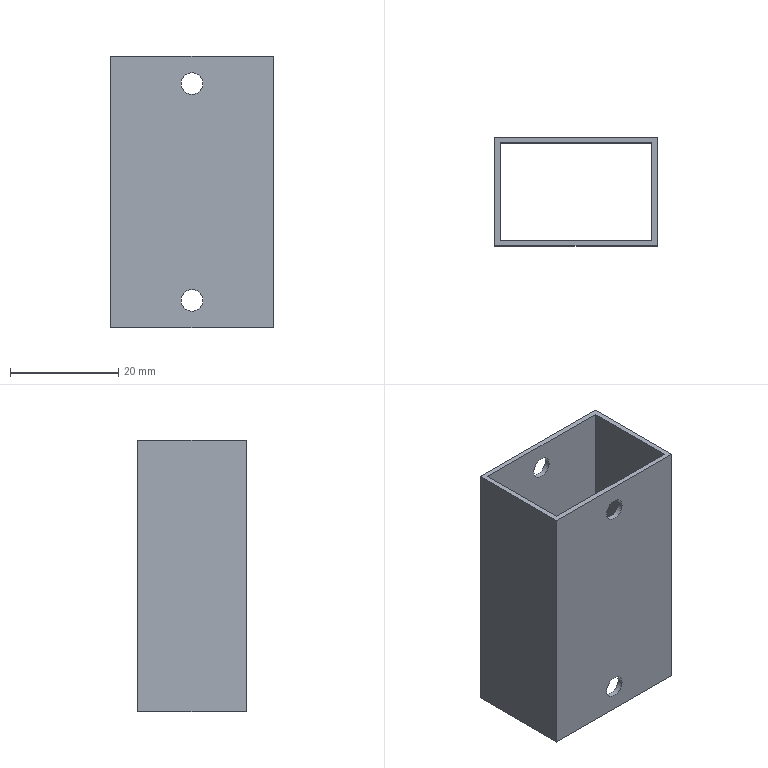Part | SolidWorks | features BaseBody 1 | 1 solid | 18 faces | box 30 x 20 x 50 mm | volume 4750 mm3 | plane 10 | cylinder 8 | commonest cylinder face diameters 4 x8
STEP:
#1=CARTESIAN_POINT('',(-2.,-10.,-20.));
#2=VERTEX_POINT('',#1);
#3=CARTESIAN_POINT('',(2.,-10.,-20.));
#4=VERTEX_POINT('',#3);
#5=CARTESIAN_POINT('',(0.,-10.,-20.));
#6=DIRECTION('',(0.,-1.,0.));
#7=DIRECTION('',(-1.,0.,0.));
#8=AXIS2_PLACEMENT_3D('',#5,#6,#7);
#9=CIRCLE('',#8,2.);
#10=EDGE_CURVE('',#2,#4,#9,.T.);
#11=ORIENTED_EDGE('',*,*,#10,.T.);
#12=CARTESIAN_POINT('',(2.,-9.,-20.));
#13=VERTEX_POINT('',#12);
#14=CARTESIAN_POINT('',(2.,-20.,-20.));
#15=DIRECTION('',(0.,1.,0.));
#16=VECTOR('',#15,1000.);
#17=LINE('',#14,#16);
#18=EDGE_CURVE('',#4,#13,#17,.T.);
#19=ORIENTED_EDGE('',*,*,#18,.T.);
#20=CARTESIAN_POINT('',(-2.,-9.,-20.));
#21=VERTEX_POINT('',#20);
#22=CARTESIAN_POINT('',(0.,-9.,-20.));
#23=DIRECTION('',(0.,-1.,0.));
#24=DIRECTION('',(-1.,0.,0.));
#25=AXIS2_PLACEMENT_3D('',#22,#23,#24);
#26=CIRCLE('',#25,2.);
#27=EDGE_CURVE('',#21,#13,#26,.T.);
#28=ORIENTED_EDGE('',*,*,#27,.F.);
#29=CARTESIAN_POINT('',(-2.,-20.,-20.));
#30=DIRECTION('',(0.,1.,0.));
#31=VECTOR('',#30,1000.);
#32=LINE('',#29,#31);
#33=EDGE_CURVE('',#2,#21,#32,.T.);
#34=ORIENTED_EDGE('',*,*,#33,.F.);
#35=EDGE_LOOP('',(#11,#19,#28,#34));
#36=FACE_OUTER_BOUND('',#35,.T.);
#37=CARTESIAN_POINT('',(0.,-20.,-20.));
#38=DIRECTION('',(0.,1.,0.));
#39=DIRECTION('',(-1.,0.,0.));
#40=AXIS2_PLACEMENT_3D('',#37,#38,#39);
#41=CYLINDRICAL_SURFACE('',#40,2.);
#42=ADVANCED_FACE('',(#36),#41,.F.);
#43=CARTESIAN_POINT('',(-2.,-10.,20.));
#44=VERTEX_POINT('',#43);
#45=CARTESIAN_POINT('',(2.,-10.,20.));
#46=VERTEX_POINT('',#45);
#47=CARTESIAN_POINT('',(0.,-10.,20.));
#48=DIRECTION('',(0.,-1.,0.));
#49=DIRECTION('',(-1.,0.,0.));
#50=AXIS2_PLACEMENT_3D('',#47,#48,#49);
#51=CIRCLE('',#50,2.);
#52=EDGE_CURVE('',#44,#46,#51,.T.);
#53=ORIENTED_EDGE('',*,*,#52,.T.);
#54=CARTESIAN_POINT('',(2.,-9.,20.));
#55=VERTEX_POINT('',#54);
#56=CARTESIAN_POINT('',(2.,-20.,20.));
#57=DIRECTION('',(0.,1.,0.));
#58=VECTOR('',#57,1000.);
#59=LINE('',#56,#58);
#60=EDGE_CURVE('',#46,#55,#59,.T.);
#61=ORIENTED_EDGE('',*,*,#60,.T.);
#62=CARTESIAN_POINT('',(-2.,-9.,20.));
#63=VERTEX_POINT('',#62);
#64=CARTESIAN_POINT('',(0.,-9.,20.));
#65=DIRECTION('',(0.,-1.,0.));
#66=DIRECTION('',(-1.,0.,0.));
#67=AXIS2_PLACEMENT_3D('',#64,#65,#66);
#68=CIRCLE('',#67,2.);
#69=EDGE_CURVE('',#63,#55,#68,.T.);
#70=ORIENTED_EDGE('',*,*,#69,.F.);
#71=CARTESIAN_POINT('',(-2.,-20.,20.));
#72=DIRECTION('',(0.,1.,0.));
#73=VECTOR('',#72,1000.);
#74=LINE('',#71,#73);
#75=EDGE_CURVE('',#44,#63,#74,.T.);
#76=ORIENTED_EDGE('',*,*,#75,.F.);
#77=EDGE_LOOP('',(#53,#61,#70,#76));
#78=FACE_OUTER_BOUND('',#77,.T.);
#79=CARTESIAN_POINT('',(0.,-20.,20.));
#80=DIRECTION('',(0.,1.,0.));
#81=DIRECTION('',(-1.,0.,0.));
#82=AXIS2_PLACEMENT_3D('',#79,#80,#81);
#83=CYLINDRICAL_SURFACE('',#82,2.);
#84=ADVANCED_FACE('',(#78),#83,.F.);
#85=CARTESIAN_POINT('',(2.,9.,-20.));
#86=VERTEX_POINT('',#85);
#87=CARTESIAN_POINT('',(-2.,9.,-20.));
#88=VERTEX_POINT('',#87);
#89=CARTESIAN_POINT('',(0.,9.,-20.));
#90=DIRECTION('',(0.,1.,0.));
#91=DIRECTION('',(-1.,0.,0.));
#92=AXIS2_PLACEMENT_3D('',#89,#90,#91);
#93=CIRCLE('',#92,2.);
#94=EDGE_CURVE('',#86,#88,#93,.T.);
#95=ORIENTED_EDGE('',*,*,#94,.F.);
#96=CARTESIAN_POINT('',(2.,10.,-20.));
#97=VERTEX_POINT('',#96);
#98=CARTESIAN_POINT('',(2.,-20.,-20.));
#99=DIRECTION('',(0.,1.,0.));
#100=VECTOR('',#99,1000.);
#101=LINE('',#98,#100);
#102=EDGE_CURVE('',#86,#97,#101,.T.);
#103=ORIENTED_EDGE('',*,*,#102,.T.);
#104=CARTESIAN_POINT('',(-2.,10.,-20.));
#105=VERTEX_POINT('',#104);
#106=CARTESIAN_POINT('',(0.,10.,-20.));
#107=DIRECTION('',(0.,1.,0.));
#108=DIRECTION('',(-1.,0.,0.));
#109=AXIS2_PLACEMENT_3D('',#106,#107,#108);
#110=CIRCLE('',#109,2.);
#111=EDGE_CURVE('',#97,#105,#110,.T.);
#112=ORIENTED_EDGE('',*,*,#111,.T.);
#113=CARTESIAN_POINT('',(-2.,-20.,-20.));
#114=DIRECTION('',(0.,1.,0.));
#115=VECTOR('',#114,1000.);
#116=LINE('',#113,#115);
#117=EDGE_CURVE('',#88,#105,#116,.T.);
#118=ORIENTED_EDGE('',*,*,#117,.F.);
#119=EDGE_LOOP('',(#95,#103,#112,#118));
#120=FACE_OUTER_BOUND('',#119,.T.);
#121=CARTESIAN_POINT('',(0.,-20.,-20.));
#122=DIRECTION('',(0.,1.,0.));
#123=DIRECTION('',(-1.,0.,0.));
#124=AXIS2_PLACEMENT_3D('',#121,#122,#123);
#125=CYLINDRICAL_SURFACE('',#124,2.);
#126=ADVANCED_FACE('',(#120),#125,.F.);
#127=CARTESIAN_POINT('',(2.,9.,20.));
#128=VERTEX_POINT('',#127);
#129=CARTESIAN_POINT('',(-2.,9.,20.));
#130=VERTEX_POINT('',#129);
#131=CARTESIAN_POINT('',(0.,9.,20.));
#132=DIRECTION('',(0.,1.,0.));
#133=DIRECTION('',(-1.,0.,0.));
#134=AXIS2_PLACEMENT_3D('',#131,#132,#133);
#135=CIRCLE('',#134,2.);
#136=EDGE_CURVE('',#128,#130,#135,.T.);
#137=ORIENTED_EDGE('',*,*,#136,.F.);
#138=CARTESIAN_POINT('',(2.,10.,20.));
#139=VERTEX_POINT('',#138);
#140=CARTESIAN_POINT('',(2.,-20.,20.));
#141=DIRECTION('',(0.,1.,0.));
#142=VECTOR('',#141,1000.);
#143=LINE('',#140,#142);
#144=EDGE_CURVE('',#128,#139,#143,.T.);
#145=ORIENTED_EDGE('',*,*,#144,.T.);
#146=CARTESIAN_POINT('',(-2.,10.,20.));
#147=VERTEX_POINT('',#146);
#148=CARTESIAN_POINT('',(0.,10.,20.));
#149=DIRECTION('',(0.,1.,0.));
#150=DIRECTION('',(-1.,0.,0.));
#151=AXIS2_PLACEMENT_3D('',#148,#149,#150);
#152=CIRCLE('',#151,2.);
#153=EDGE_CURVE('',#139,#147,#152,.T.);
#154=ORIENTED_EDGE('',*,*,#153,.T.);
#155=CARTESIAN_POINT('',(-2.,-20.,20.));
#156=DIRECTION('',(0.,1.,0.));
#157=VECTOR('',#156,1000.);
#158=LINE('',#155,#157);
#159=EDGE_CURVE('',#130,#147,#158,.T.);
#160=ORIENTED_EDGE('',*,*,#159,.F.);
#161=EDGE_LOOP('',(#137,#145,#154,#160));
#162=FACE_OUTER_BOUND('',#161,.T.);
#163=CARTESIAN_POINT('',(0.,-20.,20.));
#164=DIRECTION('',(0.,1.,0.));
#165=DIRECTION('',(-1.,0.,0.));
#166=AXIS2_PLACEMENT_3D('',#163,#164,#165);
#167=CYLINDRICAL_SURFACE('',#166,2.);
#168=ADVANCED_FACE('',(#162),#167,.F.);
#169=CARTESIAN_POINT('',(15.,-10.,25.));
#170=VERTEX_POINT('',#169);
#171=CARTESIAN_POINT('',(15.,-10.,-25.));
#172=VERTEX_POINT('',#171);
#173=CARTESIAN_POINT('',(15.,-10.,25.));
#174=DIRECTION('',(0.,0.,-1.));
#175=VECTOR('',#174,1000.);
#176=LINE('',#173,#175);
#177=EDGE_CURVE('',#170,#172,#176,.T.);
#178=ORIENTED_EDGE('',*,*,#177,.F.);
#179=CARTESIAN_POINT('',(-15.,-10.,25.));
#180=VERTEX_POINT('',#179);
#181=CARTESIAN_POINT('',(15.,-10.,25.));
#182=DIRECTION('',(1.,0.,0.));
#183=VECTOR('',#182,1000.);
#184=LINE('',#181,#183);
#185=EDGE_CURVE('',#180,#170,#184,.T.);
#186=ORIENTED_EDGE('',*,*,#185,.F.);
#187=CARTESIAN_POINT('',(-15.,-10.,-25.));
#188=VERTEX_POINT('',#187);
#189=CARTESIAN_POINT('',(-15.,-10.,25.));
#190=DIRECTION('',(0.,0.,1.));
#191=VECTOR('',#190,1000.);
#192=LINE('',#189,#191);
#193=EDGE_CURVE('',#188,#180,#192,.T.);
#194=ORIENTED_EDGE('',*,*,#193,.F.);
#195=CARTESIAN_POINT('',(15.,-10.,-25.));
#196=DIRECTION('',(-1.,0.,0.));
#197=VECTOR('',#196,1000.);
#198=LINE('',#195,#197);
#199=EDGE_CURVE('',#172,#188,#198,.T.);
#200=ORIENTED_EDGE('',*,*,#199,.F.);
#201=EDGE_LOOP('',(#178,#186,#194,#200));
#202=FACE_OUTER_BOUND('',#201,.T.);
#203=ORIENTED_EDGE('',*,*,#10,.F.);
#204=CARTESIAN_POINT('',(0.,-10.,-20.));
#205=DIRECTION('',(0.,-1.,0.));
#206=DIRECTION('',(-1.,0.,0.));
#207=AXIS2_PLACEMENT_3D('',#204,#205,#206);
#208=CIRCLE('',#207,2.);
#209=EDGE_CURVE('',#4,#2,#208,.T.);
#210=ORIENTED_EDGE('',*,*,#209,.F.);
#211=EDGE_LOOP('',(#203,#210));
#212=FACE_BOUND('',#211,.T.);
#213=ORIENTED_EDGE('',*,*,#52,.F.);
#214=CARTESIAN_POINT('',(0.,-10.,20.));
#215=DIRECTION('',(0.,-1.,0.));
#216=DIRECTION('',(-1.,0.,0.));
#217=AXIS2_PLACEMENT_3D('',#214,#215,#216);
#218=CIRCLE('',#217,2.);
#219=EDGE_CURVE('',#46,#44,#218,.T.);
#220=ORIENTED_EDGE('',*,*,#219,.F.);
#221=EDGE_LOOP('',(#213,#220));
#222=FACE_BOUND('',#221,.T.);
#223=CARTESIAN_POINT('',(15.,-10.,25.));
#224=DIRECTION('',(0.,1.,0.));
#225=DIRECTION('',(0.,0.,1.));
#226=AXIS2_PLACEMENT_3D('',#223,#224,#225);
#227=PLANE('',#226);
#228=ADVANCED_FACE('',(#202,#212,#222),#227,.F.);
#229=CARTESIAN_POINT('',(-14.,9.,-25.));
#230=VERTEX_POINT('',#229);
#231=CARTESIAN_POINT('',(14.,9.,-25.));
#232=VERTEX_POINT('',#231);
#233=CARTESIAN_POINT('',(0.,9.,-25.));
#234=DIRECTION('',(1.,0.,0.));
#235=VECTOR('',#234,1000.);
#236=LINE('',#233,#235);
#237=EDGE_CURVE('',#230,#232,#236,.T.);
#238=ORIENTED_EDGE('',*,*,#237,.F.);
#239=CARTESIAN_POINT('',(-14.,-9.,-25.));
#240=VERTEX_POINT('',#239);
#241=CARTESIAN_POINT('',(-14.,0.,-25.));
#242=DIRECTION('',(0.,1.,0.));
#243=VECTOR('',#242,1000.);
#244=LINE('',#241,#243);
#245=EDGE_CURVE('',#240,#230,#244,.T.);
#246=ORIENTED_EDGE('',*,*,#245,.F.);
#247=CARTESIAN_POINT('',(14.,-9.,-25.));
#248=VERTEX_POINT('',#247);
#249=CARTESIAN_POINT('',(0.,-9.,-25.));
#250=DIRECTION('',(-1.,0.,0.));
#251=VECTOR('',#250,1000.);
#252=LINE('',#249,#251);
#253=EDGE_CURVE('',#248,#240,#252,.T.);
#254=ORIENTED_EDGE('',*,*,#253,.F.);
#255=CARTESIAN_POINT('',(14.,0.,-25.));
#256=DIRECTION('',(0.,-1.,0.));
#257=VECTOR('',#256,1000.);
#258=LINE('',#255,#257);
#259=EDGE_CURVE('',#232,#248,#258,.T.);
#260=ORIENTED_EDGE('',*,*,#259,.F.);
#261=EDGE_LOOP('',(#238,#246,#254,#260));
#262=FACE_BOUND('',#261,.T.);
#263=CARTESIAN_POINT('',(15.,10.,-25.));
#264=VERTEX_POINT('',#263);
#265=CARTESIAN_POINT('',(-15.,10.,-25.));
#266=VERTEX_POINT('',#265);
#267=CARTESIAN_POINT('',(0.,10.,-25.));
#268=DIRECTION('',(-1.,0.,0.));
#269=VECTOR('',#268,1000.);
#270=LINE('',#267,#269);
#271=EDGE_CURVE('',#264,#266,#270,.T.);
#272=ORIENTED_EDGE('',*,*,#271,.F.);
#273=CARTESIAN_POINT('',(15.,0.,-25.));
#274=DIRECTION('',(0.,1.,0.));
#275=VECTOR('',#274,1000.);
#276=LINE('',#273,#275);
#277=EDGE_CURVE('',#172,#264,#276,.T.);
#278=ORIENTED_EDGE('',*,*,#277,.F.);
#279=ORIENTED_EDGE('',*,*,#199,.T.);
#280=CARTESIAN_POINT('',(-15.,0.,-25.));
#281=DIRECTION('',(0.,-1.,0.));
#282=VECTOR('',#281,1000.);
#283=LINE('',#280,#282);
#284=EDGE_CURVE('',#266,#188,#283,.T.);
#285=ORIENTED_EDGE('',*,*,#284,.F.);
#286=EDGE_LOOP('',(#272,#278,#279,#285));
#287=FACE_OUTER_BOUND('',#286,.T.);
#288=CARTESIAN_POINT('',(0.,0.,-25.));
#289=DIRECTION('',(0.,0.,1.));
#290=DIRECTION('',(1.,0.,0.));
#291=AXIS2_PLACEMENT_3D('',#288,#289,#290);
#292=PLANE('',#291);
#293=ADVANCED_FACE('',(#262,#287),#292,.F.);
#294=CARTESIAN_POINT('',(15.,10.,25.));
#295=VERTEX_POINT('',#294);
#296=CARTESIAN_POINT('',(15.,10.,25.));
#297=DIRECTION('',(0.,0.,-1.));
#298=VECTOR('',#297,1000.);
#299=LINE('',#296,#298);
#300=EDGE_CURVE('',#295,#264,#299,.T.);
#301=ORIENTED_EDGE('',*,*,#300,.F.);
#302=CARTESIAN_POINT('',(15.,-10.,25.));
#303=DIRECTION('',(0.,1.,0.));
#304=VECTOR('',#303,1000.);
#305=LINE('',#302,#304);
#306=EDGE_CURVE('',#170,#295,#305,.T.);
#307=ORIENTED_EDGE('',*,*,#306,.F.);
#308=ORIENTED_EDGE('',*,*,#177,.T.);
#309=ORIENTED_EDGE('',*,*,#277,.T.);
#310=EDGE_LOOP('',(#301,#307,#308,#309));
#311=FACE_OUTER_BOUND('',#310,.T.);
#312=CARTESIAN_POINT('',(15.,-10.,25.));
#313=DIRECTION('',(-1.,0.,0.));
#314=DIRECTION('',(0.,-1.,0.));
#315=AXIS2_PLACEMENT_3D('',#312,#313,#314);
#316=PLANE('',#315);
#317=ADVANCED_FACE('',(#311),#316,.F.);
#318=CARTESIAN_POINT('',(14.,-9.,25.));
#319=VERTEX_POINT('',#318);
#320=CARTESIAN_POINT('',(-14.,-9.,25.));
#321=VERTEX_POINT('',#320);
#322=CARTESIAN_POINT('',(0.,-9.,25.));
#323=DIRECTION('',(-1.,0.,0.));
#324=VECTOR('',#323,1000.);
#325=LINE('',#322,#324);
#326=EDGE_CURVE('',#319,#321,#325,.T.);
#327=ORIENTED_EDGE('',*,*,#326,.T.);
#328=CARTESIAN_POINT('',(-14.,9.,25.));
#329=VERTEX_POINT('',#328);
#330=CARTESIAN_POINT('',(-14.,0.,25.));
#331=DIRECTION('',(0.,1.,0.));
#332=VECTOR('',#331,1000.);
#333=LINE('',#330,#332);
#334=EDGE_CURVE('',#321,#329,#333,.T.);
#335=ORIENTED_EDGE('',*,*,#334,.T.);
#336=CARTESIAN_POINT('',(14.,9.,25.));
#337=VERTEX_POINT('',#336);
#338=CARTESIAN_POINT('',(0.,9.,25.));
#339=DIRECTION('',(1.,0.,0.));
#340=VECTOR('',#339,1000.);
#341=LINE('',#338,#340);
#342=EDGE_CURVE('',#329,#337,#341,.T.);
#343=ORIENTED_EDGE('',*,*,#342,.T.);
#344=CARTESIAN_POINT('',(14.,0.,25.));
#345=DIRECTION('',(0.,-1.,0.));
#346=VECTOR('',#345,1000.);
#347=LINE('',#344,#346);
#348=EDGE_CURVE('',#337,#319,#347,.T.);
#349=ORIENTED_EDGE('',*,*,#348,.T.);
#350=EDGE_LOOP('',(#327,#335,#343,#349));
#351=FACE_BOUND('',#350,.T.);
#352=ORIENTED_EDGE('',*,*,#306,.T.);
#353=CARTESIAN_POINT('',(-15.,10.,25.));
#354=VERTEX_POINT('',#353);
#355=CARTESIAN_POINT('',(0.,10.,25.));
#356=DIRECTION('',(-1.,0.,0.));
#357=VECTOR('',#356,1000.);
#358=LINE('',#355,#357);
#359=EDGE_CURVE('',#295,#354,#358,.T.);
#360=ORIENTED_EDGE('',*,*,#359,.T.);
#361=CARTESIAN_POINT('',(-15.,0.,25.));
#362=DIRECTION('',(0.,-1.,0.));
#363=VECTOR('',#362,1000.);
#364=LINE('',#361,#363);
#365=EDGE_CURVE('',#354,#180,#364,.T.);
#366=ORIENTED_EDGE('',*,*,#365,.T.);
#367=ORIENTED_EDGE('',*,*,#185,.T.);
#368=EDGE_LOOP('',(#352,#360,#366,#367));
#369=FACE_OUTER_BOUND('',#368,.T.);
#370=CARTESIAN_POINT('',(0.,0.,25.));
#371=DIRECTION('',(0.,0.,1.));
#372=DIRECTION('',(1.,0.,0.));
#373=AXIS2_PLACEMENT_3D('',#370,#371,#372);
#374=PLANE('',#373);
#375=ADVANCED_FACE('',(#351,#369),#374,.T.);
#376=ORIENTED_EDGE('',*,*,#193,.T.);
#377=ORIENTED_EDGE('',*,*,#365,.F.);
#378=CARTESIAN_POINT('',(-15.,10.,25.));
#379=DIRECTION('',(0.,0.,1.));
#380=VECTOR('',#379,1000.);
#381=LINE('',#378,#380);
#382=EDGE_CURVE('',#266,#354,#381,.T.);
#383=ORIENTED_EDGE('',*,*,#382,.F.);
#384=ORIENTED_EDGE('',*,*,#284,.T.);
#385=EDGE_LOOP('',(#376,#377,#383,#384));
#386=FACE_OUTER_BOUND('',#385,.T.);
#387=CARTESIAN_POINT('',(-15.,-10.,25.));
#388=DIRECTION('',(1.,0.,0.));
#389=DIRECTION('',(0.,0.,-1.));
#390=AXIS2_PLACEMENT_3D('',#387,#388,#389);
#391=PLANE('',#390);
#392=ADVANCED_FACE('',(#386),#391,.F.);
#393=ORIENTED_EDGE('',*,*,#18,.F.);
#394=ORIENTED_EDGE('',*,*,#209,.T.);
#395=ORIENTED_EDGE('',*,*,#33,.T.);
#396=CARTESIAN_POINT('',(0.,-9.,-20.));
#397=DIRECTION('',(0.,-1.,0.));
#398=DIRECTION('',(-1.,0.,0.));
#399=AXIS2_PLACEMENT_3D('',#396,#397,#398);
#400=CIRCLE('',#399,2.);
#401=EDGE_CURVE('',#13,#21,#400,.T.);
#402=ORIENTED_EDGE('',*,*,#401,.F.);
#403=EDGE_LOOP('',(#393,#394,#395,#402));
#404=FACE_OUTER_BOUND('',#403,.T.);
#405=CARTESIAN_POINT('',(0.,-20.,-20.));
#406=DIRECTION('',(0.,1.,0.));
#407=DIRECTION('',(-1.,0.,0.));
#408=AXIS2_PLACEMENT_3D('',#405,#406,#407);
#409=CYLINDRICAL_SURFACE('',#408,2.);
#410=ADVANCED_FACE('',(#404),#409,.F.);
#411=ORIENTED_EDGE('',*,*,#60,.F.);
#412=ORIENTED_EDGE('',*,*,#219,.T.);
#413=ORIENTED_EDGE('',*,*,#75,.T.);
#414=CARTESIAN_POINT('',(0.,-9.,20.));
#415=DIRECTION('',(0.,-1.,0.));
#416=DIRECTION('',(-1.,0.,0.));
#417=AXIS2_PLACEMENT_3D('',#414,#415,#416);
#418=CIRCLE('',#417,2.);
#419=EDGE_CURVE('',#55,#63,#418,.T.);
#420=ORIENTED_EDGE('',*,*,#419,.F.);
#421=EDGE_LOOP('',(#411,#412,#413,#420));
#422=FACE_OUTER_BOUND('',#421,.T.);
#423=CARTESIAN_POINT('',(0.,-20.,20.));
#424=DIRECTION('',(0.,1.,0.));
#425=DIRECTION('',(-1.,0.,0.));
#426=AXIS2_PLACEMENT_3D('',#423,#424,#425);
#427=CYLINDRICAL_SURFACE('',#426,2.);
#428=ADVANCED_FACE('',(#422),#427,.F.);
#429=ORIENTED_EDGE('',*,*,#348,.F.);
#430=CARTESIAN_POINT('',(14.,9.,25.));
#431=DIRECTION('',(0.,0.,-1.));
#432=VECTOR('',#431,1000.);
#433=LINE('',#430,#432);
#434=EDGE_CURVE('',#337,#232,#433,.T.);
#435=ORIENTED_EDGE('',*,*,#434,.T.);
#436=ORIENTED_EDGE('',*,*,#259,.T.);
#437=CARTESIAN_POINT('',(14.,-9.,25.));
#438=DIRECTION('',(0.,0.,1.));
#439=VECTOR('',#438,1000.);
#440=LINE('',#437,#439);
#441=EDGE_CURVE('',#248,#319,#440,.T.);
#442=ORIENTED_EDGE('',*,*,#441,.T.);
#443=EDGE_LOOP('',(#429,#435,#436,#442));
#444=FACE_OUTER_BOUND('',#443,.T.);
#445=CARTESIAN_POINT('',(14.,-9.,25.));
#446=DIRECTION('',(-1.,0.,0.));
#447=DIRECTION('',(0.,0.,1.));
#448=AXIS2_PLACEMENT_3D('',#445,#446,#447);
#449=PLANE('',#448);
#450=ADVANCED_FACE('',(#444),#449,.T.);
#451=ORIENTED_EDGE('',*,*,#342,.F.);
#452=CARTESIAN_POINT('',(-14.,9.,25.));
#453=DIRECTION('',(0.,0.,-1.));
#454=VECTOR('',#453,1000.);
#455=LINE('',#452,#454);
#456=EDGE_CURVE('',#329,#230,#455,.T.);
#457=ORIENTED_EDGE('',*,*,#456,.T.);
#458=ORIENTED_EDGE('',*,*,#237,.T.);
#459=ORIENTED_EDGE('',*,*,#434,.F.);
#460=EDGE_LOOP('',(#451,#457,#458,#459));
#461=FACE_OUTER_BOUND('',#460,.T.);
#462=CARTESIAN_POINT('',(0.,9.,-20.));
#463=DIRECTION('',(0.,1.,0.));
#464=DIRECTION('',(-1.,0.,0.));
#465=AXIS2_PLACEMENT_3D('',#462,#463,#464);
#466=CIRCLE('',#465,2.);
#467=EDGE_CURVE('',#88,#86,#466,.T.);
#468=ORIENTED_EDGE('',*,*,#467,.T.);
#469=ORIENTED_EDGE('',*,*,#94,.T.);
#470=EDGE_LOOP('',(#468,#469));
#471=FACE_BOUND('',#470,.T.);
#472=CARTESIAN_POINT('',(0.,9.,20.));
#473=DIRECTION('',(0.,1.,0.));
#474=DIRECTION('',(-1.,0.,0.));
#475=AXIS2_PLACEMENT_3D('',#472,#473,#474);
#476=CIRCLE('',#475,2.);
#477=EDGE_CURVE('',#130,#128,#476,.T.);
#478=ORIENTED_EDGE('',*,*,#477,.T.);
#479=ORIENTED_EDGE('',*,*,#136,.T.);
#480=EDGE_LOOP('',(#478,#479));
#481=FACE_BOUND('',#480,.T.);
#482=CARTESIAN_POINT('',(14.,9.,25.));
#483=DIRECTION('',(0.,-1.,0.));
#484=DIRECTION('',(0.,0.,-1.));
#485=AXIS2_PLACEMENT_3D('',#482,#483,#484);
#486=PLANE('',#485);
#487=ADVANCED_FACE('',(#461,#471,#481),#486,.T.);
#488=ORIENTED_EDGE('',*,*,#334,.F.);
#489=CARTESIAN_POINT('',(-14.,-9.,25.));
#490=DIRECTION('',(0.,0.,-1.));
#491=VECTOR('',#490,1000.);
#492=LINE('',#489,#491);
#493=EDGE_CURVE('',#321,#240,#492,.T.);
#494=ORIENTED_EDGE('',*,*,#493,.T.);
#495=ORIENTED_EDGE('',*,*,#245,.T.);
#496=ORIENTED_EDGE('',*,*,#456,.F.);
#497=EDGE_LOOP('',(#488,#494,#495,#496));
#498=FACE_OUTER_BOUND('',#497,.T.);
#499=CARTESIAN_POINT('',(-14.,-9.,25.));
#500=DIRECTION('',(1.,0.,0.));
#501=DIRECTION('',(0.,1.,0.));
#502=AXIS2_PLACEMENT_3D('',#499,#500,#501);
#503=PLANE('',#502);
#504=ADVANCED_FACE('',(#498),#503,.T.);
#505=ORIENTED_EDGE('',*,*,#326,.F.);
#506=ORIENTED_EDGE('',*,*,#441,.F.);
#507=ORIENTED_EDGE('',*,*,#253,.T.);
#508=ORIENTED_EDGE('',*,*,#493,.F.);
#509=EDGE_LOOP('',(#505,#506,#507,#508));
#510=FACE_OUTER_BOUND('',#509,.T.);
#511=ORIENTED_EDGE('',*,*,#27,.T.);
#512=ORIENTED_EDGE('',*,*,#401,.T.);
#513=EDGE_LOOP('',(#511,#512));
#514=FACE_BOUND('',#513,.T.);
#515=ORIENTED_EDGE('',*,*,#69,.T.);
#516=ORIENTED_EDGE('',*,*,#419,.T.);
#517=EDGE_LOOP('',(#515,#516));
#518=FACE_BOUND('',#517,.T.);
#519=CARTESIAN_POINT('',(14.,-9.,25.));
#520=DIRECTION('',(0.,1.,0.));
#521=DIRECTION('',(0.,0.,1.));
#522=AXIS2_PLACEMENT_3D('',#519,#520,#521);
#523=PLANE('',#522);
#524=ADVANCED_FACE('',(#510,#514,#518),#523,.T.);
#525=ORIENTED_EDGE('',*,*,#382,.T.);
#526=ORIENTED_EDGE('',*,*,#359,.F.);
#527=ORIENTED_EDGE('',*,*,#300,.T.);
#528=ORIENTED_EDGE('',*,*,#271,.T.);
#529=EDGE_LOOP('',(#525,#526,#527,#528));
#530=FACE_OUTER_BOUND('',#529,.T.);
#531=CARTESIAN_POINT('',(0.,10.,-20.));
#532=DIRECTION('',(0.,1.,0.));
#533=DIRECTION('',(-1.,0.,0.));
#534=AXIS2_PLACEMENT_3D('',#531,#532,#533);
#535=CIRCLE('',#534,2.);
#536=EDGE_CURVE('',#105,#97,#535,.T.);
#537=ORIENTED_EDGE('',*,*,#536,.F.);
#538=ORIENTED_EDGE('',*,*,#111,.F.);
#539=EDGE_LOOP('',(#537,#538));
#540=FACE_BOUND('',#539,.T.);
#541=CARTESIAN_POINT('',(0.,10.,20.));
#542=DIRECTION('',(0.,1.,0.));
#543=DIRECTION('',(-1.,0.,0.));
#544=AXIS2_PLACEMENT_3D('',#541,#542,#543);
#545=CIRCLE('',#544,2.);
#546=EDGE_CURVE('',#147,#139,#545,.T.);
#547=ORIENTED_EDGE('',*,*,#546,.F.);
#548=ORIENTED_EDGE('',*,*,#153,.F.);
#549=EDGE_LOOP('',(#547,#548));
#550=FACE_BOUND('',#549,.T.);
#551=CARTESIAN_POINT('',(15.,10.,25.));
#552=DIRECTION('',(0.,-1.,0.));
#553=DIRECTION('',(1.,0.,0.));
#554=AXIS2_PLACEMENT_3D('',#551,#552,#553);
#555=PLANE('',#554);
#556=ADVANCED_FACE('',(#530,#540,#550),#555,.F.);
#557=ORIENTED_EDGE('',*,*,#102,.F.);
#558=ORIENTED_EDGE('',*,*,#467,.F.);
#559=ORIENTED_EDGE('',*,*,#117,.T.);
#560=ORIENTED_EDGE('',*,*,#536,.T.);
#561=EDGE_LOOP('',(#557,#558,#559,#560));
#562=FACE_OUTER_BOUND('',#561,.T.);
#563=CARTESIAN_POINT('',(0.,-20.,-20.));
#564=DIRECTION('',(0.,1.,0.));
#565=DIRECTION('',(-1.,0.,0.));
#566=AXIS2_PLACEMENT_3D('',#563,#564,#565);
#567=CYLINDRICAL_SURFACE('',#566,2.);
#568=ADVANCED_FACE('',(#562),#567,.F.);
#569=ORIENTED_EDGE('',*,*,#144,.F.);
#570=ORIENTED_EDGE('',*,*,#477,.F.);
#571=ORIENTED_EDGE('',*,*,#159,.T.);
#572=ORIENTED_EDGE('',*,*,#546,.T.);
#573=EDGE_LOOP('',(#569,#570,#571,#572));
#574=FACE_OUTER_BOUND('',#573,.T.);
#575=CARTESIAN_POINT('',(0.,-20.,20.));
#576=DIRECTION('',(0.,1.,0.));
#577=DIRECTION('',(-1.,0.,0.));
#578=AXIS2_PLACEMENT_3D('',#575,#576,#577);
#579=CYLINDRICAL_SURFACE('',#578,2.);
#580=ADVANCED_FACE('',(#574),#579,.F.);
#581=CLOSED_SHELL('',(#42,#84,#126,#168,#228,#293,#317,#375,#392,#410,#428,#450,#487,#504,#524,#556,#568,#580));
#582=MANIFOLD_SOLID_BREP('',#581);
#583=CARTESIAN_POINT('',(0.,0.,0.));
#584=DIRECTION('',(0.,0.,1.));
#585=DIRECTION('',(1.,0.,0.));
#586=AXIS2_PLACEMENT_3D('',#583,#584,#585);
#587=(LENGTH_UNIT()NAMED_UNIT(*)SI_UNIT(.MILLI.,.METRE.));
#588=UNCERTAINTY_MEASURE_WITH_UNIT(LENGTH_MEASURE(0.00001),#587,'','');
#589=(NAMED_UNIT(*)PLANE_ANGLE_UNIT()SI_UNIT($,.RADIAN.));
#590=(NAMED_UNIT(*)SI_UNIT($,.STERADIAN.)SOLID_ANGLE_UNIT());
#591=(GEOMETRIC_REPRESENTATION_CONTEXT(3)GLOBAL_UNCERTAINTY_ASSIGNED_CONTEXT((#588))GLOBAL_UNIT_ASSIGNED_CONTEXT((#587,#589,#590))REPRESENTATION_CONTEXT('',''));
#592=ADVANCED_BREP_SHAPE_REPRESENTATION('',(#582,#586),#591);